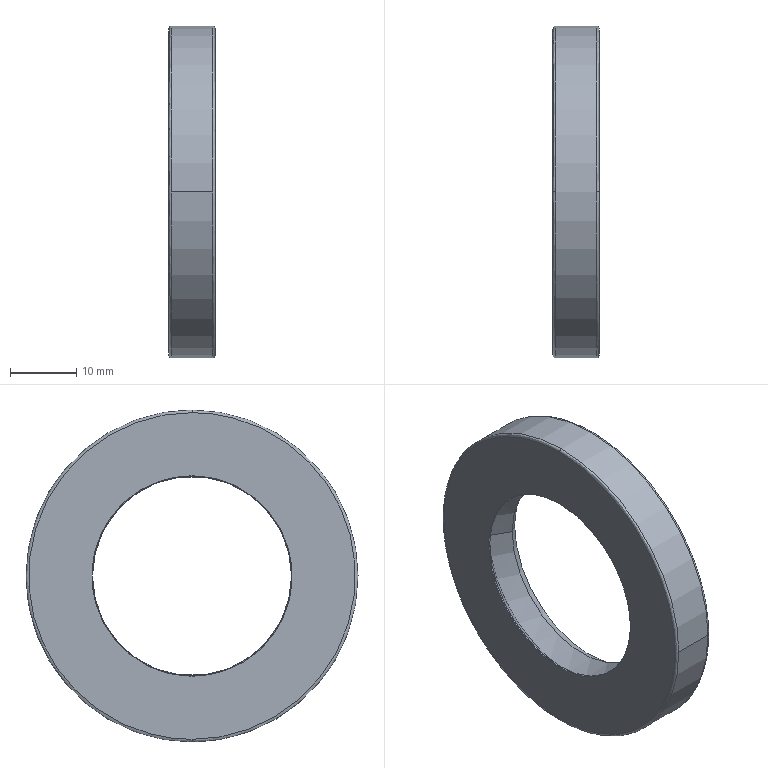Part | SolidWorks | features BaseBody 1 | 1 solid | 30 faces | box 7 x 50 x 50 mm | volume 4232 mm3 | spline 12 | cone 8 | cylinder 6 | plane 4 | commonest cylinder face diameters 34.2 x2 46.5 x2 50 x2